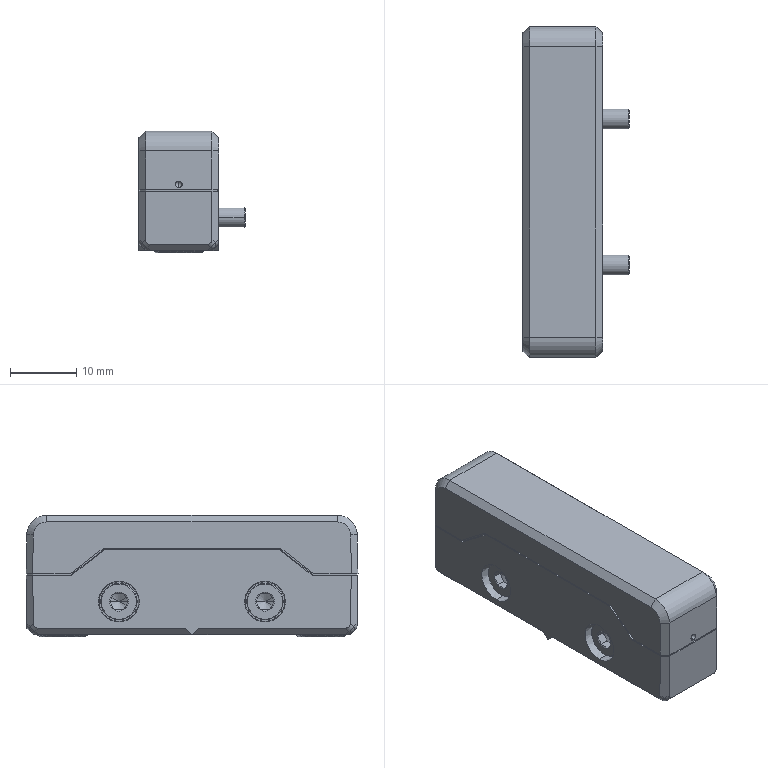Part | SolidWorks | features BaseBody 8 | 8 solids | 721 faces | box 16.002 x 50.042 x 18.313 mm | volume 6537 mm3 | plane 418 | spline 175 | cone 70 | cylinder 40 | torus 12 | sphere 6 | commonest cylinder face diameters 2.001 x12 3 x4 3.084 x4 4.975 x4 5.5 x4 6 x4